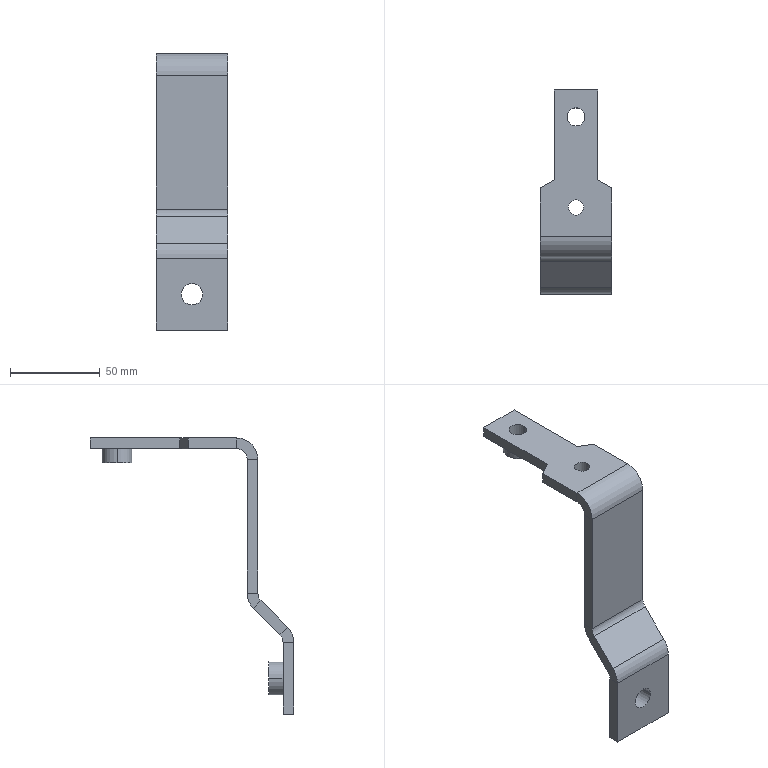Part | STEP file | 64586785 | 1 solid | 46 faces | box 40 x 113.5 x 154 mm | volume 54622 mm3 | plane 30 | cylinder 16 | commonest cylinder face diameters 12 x5 24 x3 8.5 x2 10 x2 16.5 x2 18.5 x2